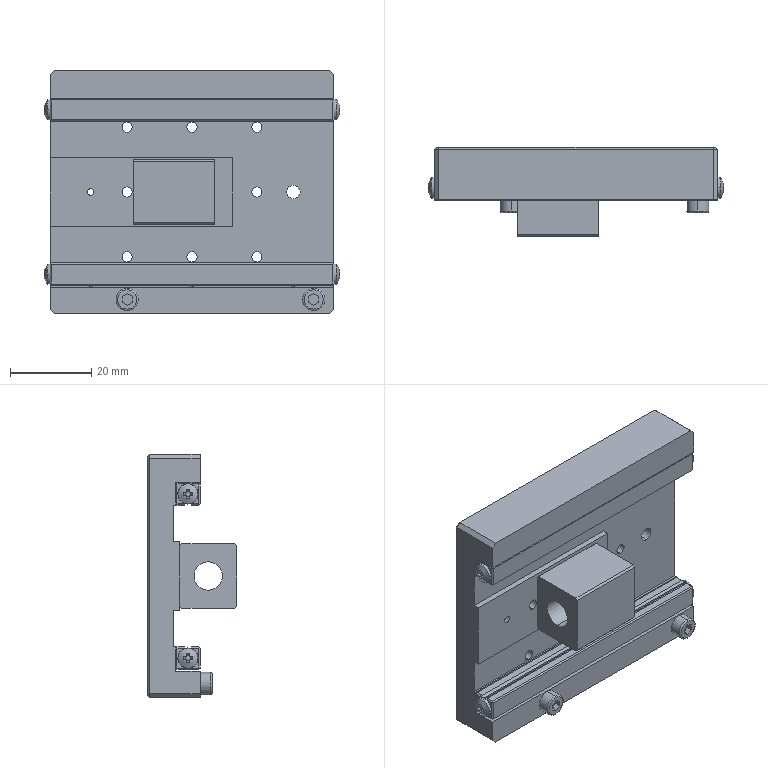Part | SolidWorks | features BaseBody 1 | 1 solid | 424 faces | box 72.934 x 22 x 60 mm | volume 41996 mm3 | plane 274 | cylinder 96 | torus 28 | cone 22 | spline 4 | commonest cylinder face diameters 2.5 x24 5.5 x20 3.3 x16 6 x16 4.5 x8 5 x8